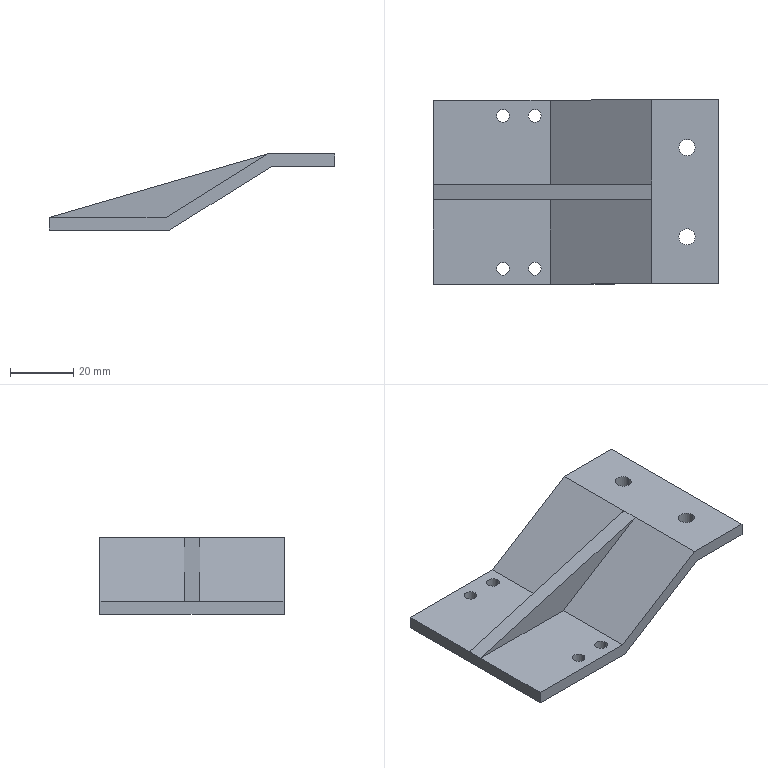Part | STEP file | Mechanical claw bracket | 1 solid | 27 faces | box 90 x 58 x 24 mm | volume 23689 mm3 | plane 15 | cylinder 12 | commonest cylinder face diameters 4 x8 5.1 x4